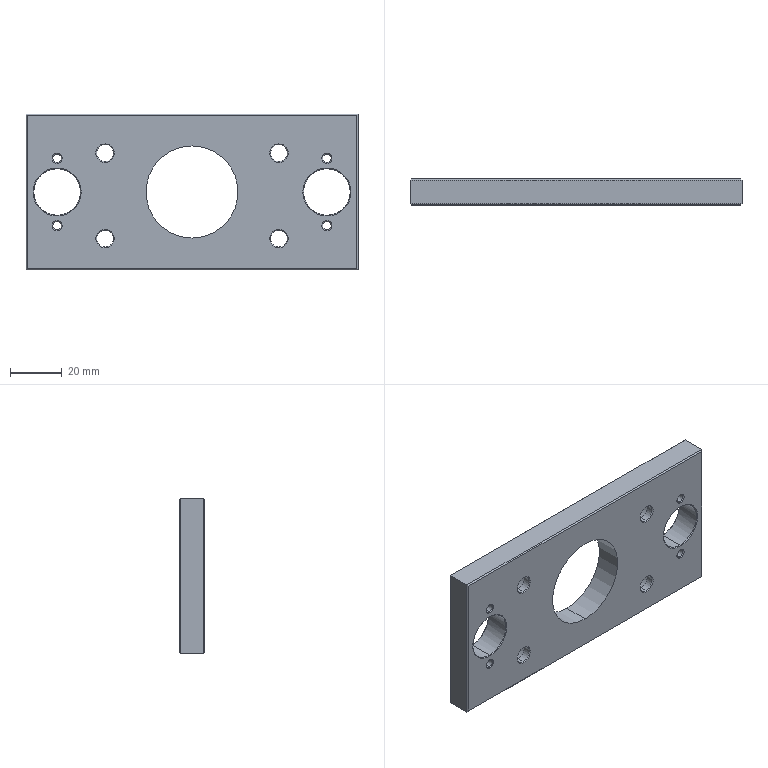Part | STEP file | 1006 | 1 solid | 88 faces | box 128 x 10 x 60 mm | volume 58293 mm3 | cone 40 | cylinder 30 | plane 18 | commonest cylinder face diameters 3.3 x8 6.5 x8 11 x8 18 x4 35.5 x2